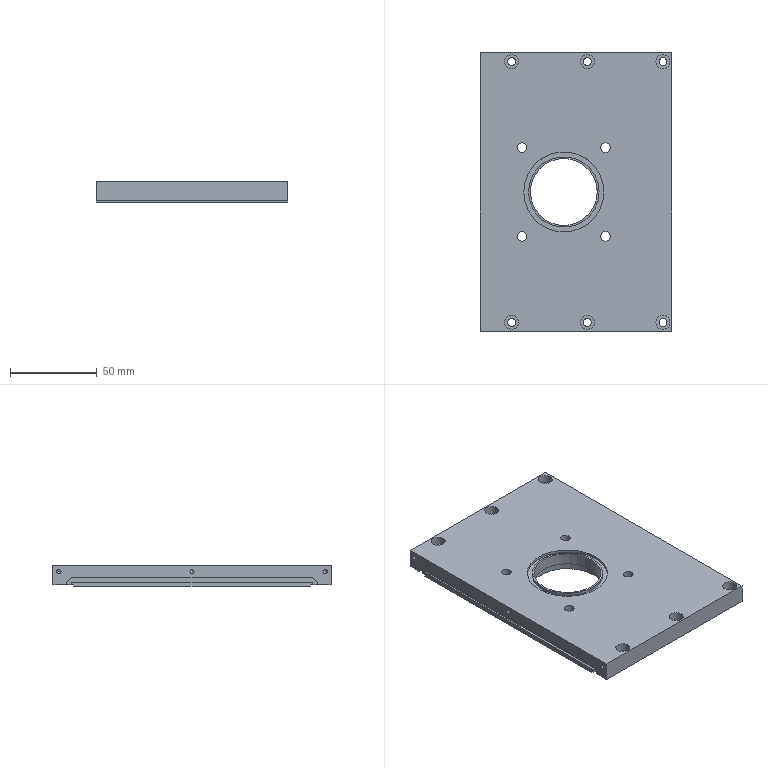Part | 1 solid | 70 faces | box 110 x 160 x 12 mm | volume 188190 mm3 | cylinder 33 | plane 31 | cone 6 | commonest cylinder face diameters 4.5 x6 8 x6 5.5 x4 2.459 x3 3.242 x3 5 x3